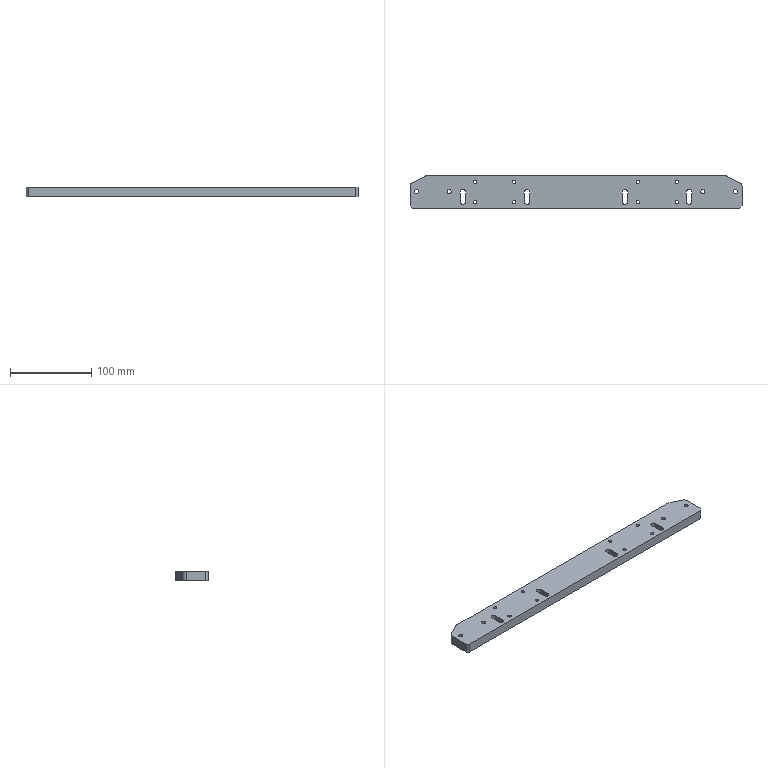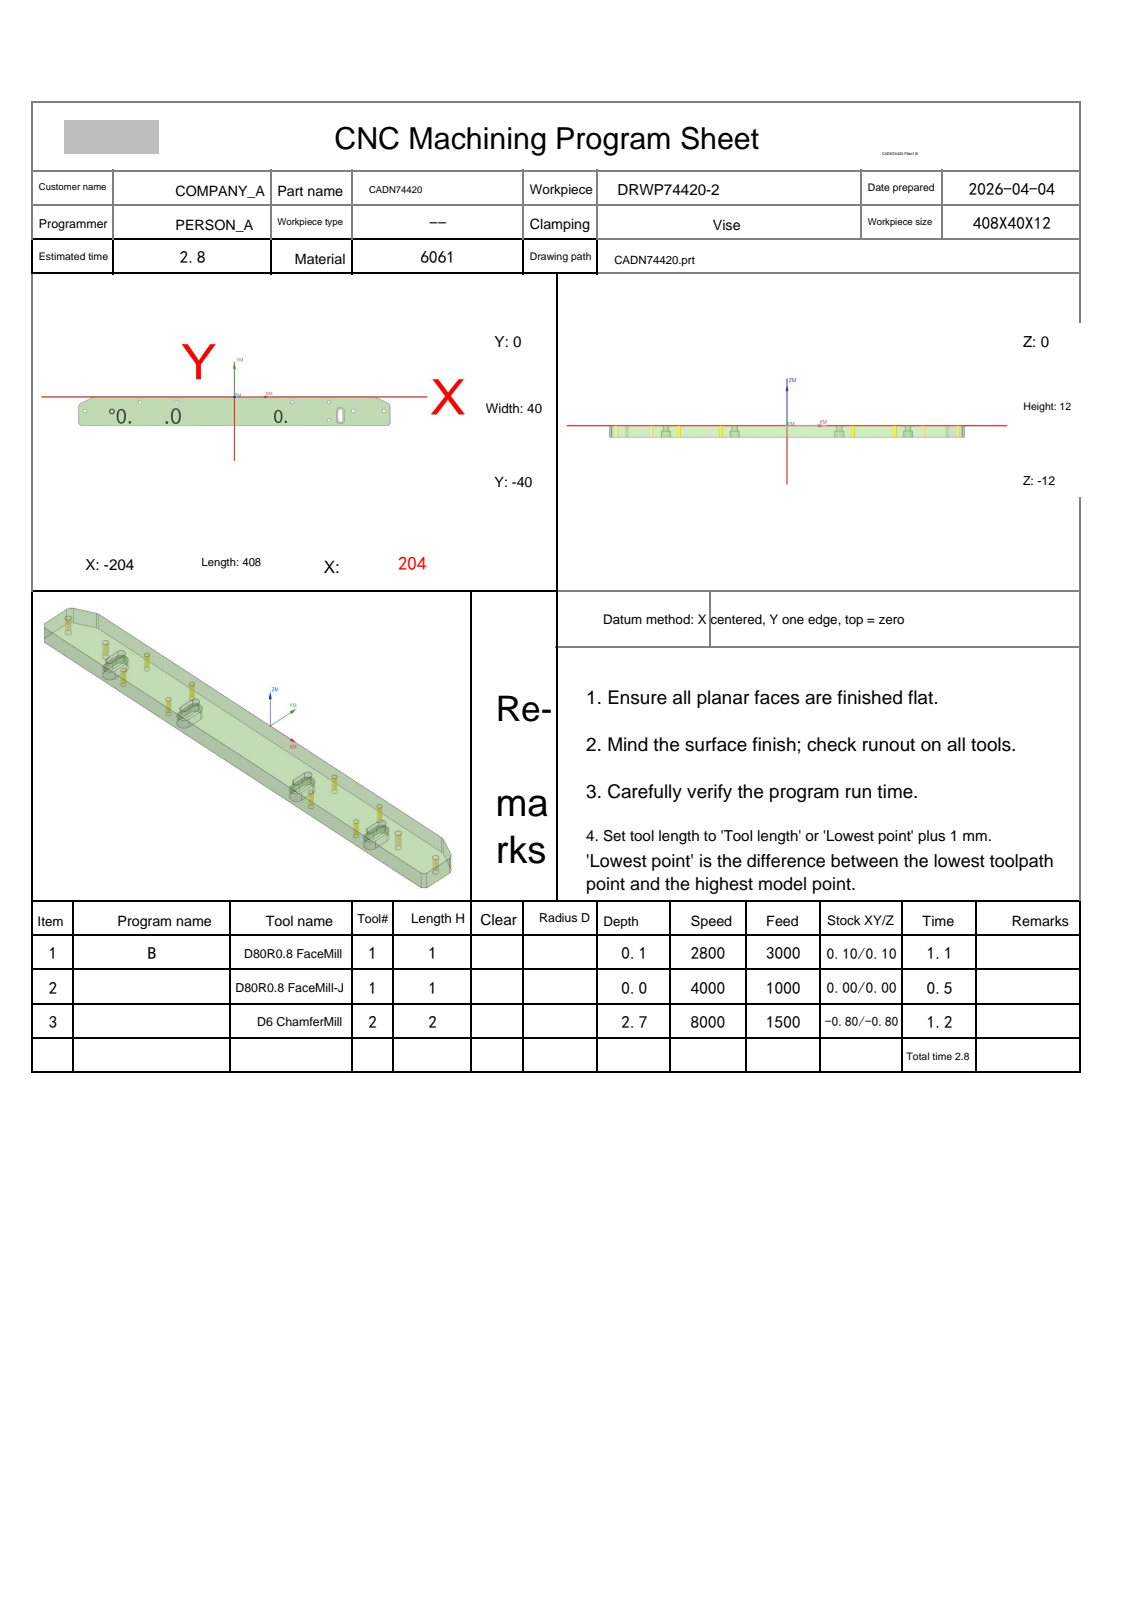NC program | NX | posted by the shop | part box 408 x 40 x 12 mm
Whole program:
%
O0001
(Machine time: 3.33 MIN)
(===Total Tool:2===)
(T1=D80R0.8 FaceMill D=80.  R=0.8  D-  H01 Z=0.    )
(T2=D6 ChamferMill   D=6.   R=0.   D-  H02 Z=-2.7  )
G80 G90 G17 G49 G40
G91 G28 Z0
M01
N1 T01 M06
(D80R0.8 FaceMill  D=80. R=0.8 H=01 ce=0.10 di=0.10)
G00 G90 G54 X-256.097 Y-20. M03 S2800
G43 H01 Z20.
M08
Z4.02
G01 Z2.02 F3000.
X-244.097
X244.097
X256.097
Z4.02
G00 X-256.097
Z3.54
G01 Z1.54
X-244.097
X244.097
X256.097
Z3.54
G00 X-256.097
Z3.06
G01 Z1.06
X-244.097
X244.097
X256.097
Z3.06
G00 X-256.097
Z2.58
G01 Z.58
X-244.097
X244.097
X256.097
Z2.58
G00 Z20.
X-256.097
Z2.1
G01 Z.1
X-244.097
X244.097
X256.097
Z2.1
G00 Z20.
G91 G28 Z0.0
M05
M09
G91 G28 Z0.0
M01
N2 T01 M06
(D80R0.8 FaceMill-J  D=80. R=0.8 H=01 ce=0.00 di=0.00)
G00 G90 G54 X-255.999 Y-20. M03 S4000
G43 H01 Z20.
M08
Z2.
G01 Z0.0 F1000.
X-243.999
X243.999
X255.999
Z2.
G00 Z20.
G91 G28 Z0.0
M05
M09
G91 G28 Z0.0
M01
N3 T02 M06
(D6 ChamferMill  D=6. R=0. H=02 ce=0.00 di=0.00)
G00 G90 G54 X-124. Y-7.5 M03 S8000
G43 H02 Z20.
M08
G98 G81 X-124. Y-7.5 Z-2.7 R3. F1000.
Y-32.5
X-76.
Y-7.5
X76.
Y-32.5
X124.
Y-7.5
G80
G00 Z20.
G00 G90 X-196.232 Y-18.63 M03 S8000
Z20.
Z-.9
G01 Z-1.4 F600.
X-196.4 Y-18.
G03 X-197.9 Y-19.5 I0.0 J-1.5
X-196. Y-21.4 I1.9 J0.0
X-194.1 Y-19.5 I0.0 J1.9
X-196. Y-17.6 I-1.9 J0.0
X-197.9 Y-19.5 I0.0 J-1.9
X-196.4 Y-21. I1.5 J0.0
G01 X-196.232 Y-20.37
Z-.9
G00 Z20.
X-156.232 Y-18.63
Z-.9
G01 Z-1.4
X-156.4 Y-18.
G03 X-157.9 Y-19.5 I0.0 J-1.5
X-156. Y-21.4 I1.9 J0.0
X-154.1 Y-19.5 I0.0 J1.9
X-156. Y-17.6 I-1.9 J0.0
X-157.9 Y-19.5 I0.0 J-1.9
X-156.4 Y-21. I1.5 J0.0
G01 X-156.232 Y-20.37
Z-.9
G00 Z20.
X155.768 Y-18.63
Z-.9
G01 Z-1.4
X155.6 Y-18.
G03 X154.1 Y-19.5 I0.0 J-1.5
X156. Y-21.4 I1.9 J0.0
X157.9 Y-19.5 I0.0 J1.9
X156. Y-17.6 I-1.9 J0.0
X154.1 Y-19.5 I0.0 J-1.9
X155.6 Y-21. I1.5 J0.0
G01 X155.768 Y-20.37
Z-.9
G00 Z20.
X195.768 Y-18.63
Z-.9
G01 Z-1.4
X195.6 Y-18.
G03 X194.1 Y-19.5 I0.0 J-1.5
X196. Y-21.4 I1.9 J0.0
X197.9 Y-19.5 I0.0 J1.9
X196. Y-17.6 I-1.9 J0.0
X194.1 Y-19.5 I0.0 J-1.9
X195.6 Y-21. I1.5 J0.0
G01 X195.768 Y-20.37
Z-.9
G00 Z20.
G00 G90 X.386 Y-41.227 M03 S6500
Z20.
Z.172
G01 Z-1.2 F1500.
G03 X.1 Y-41.027 I-1.286 J-1.532
G01 X.054 Y-40.997
X0.0 Y-41.
X-201.
X-201.259 Y-40.966
X-201.5 Y-40.866
X-201.707 Y-40.707
X-204.707 Y-37.707
X-204.866 Y-37.5
X-204.966 Y-37.259
X-205. Y-37.
Y-13.09
G02 X-201.683 Y-7.724 I6. J0.0
G01 X-185.503 Y.367
G02 X-182.82 Y1. I2.683 J-5.367
G01 X182.82
G02 X185.503 Y.367 I0.0 J-6.
G01 X201.683 Y-7.724
G02 X205. Y-13.09 I-2.683 J-5.367
G01 Y-37.
X204.966 Y-37.259
X204.866 Y-37.5
X204.707 Y-37.707
X201.707 Y-40.707
X201.5 Y-40.866
X201.259 Y-40.966
X201. Y-41.
X0.0
X-.054 Y-40.997
X-.1 Y-41.027
G03 X-.386 Y-41.227 I1. J-1.732
G01 Z.172
G00 Z10.
X-197.315 Y-19.093
Z.284
G01 Z-1.2
G03 X-197.484 Y-19.398 I1.658 J-1.118
G01 X-197.509 Y-19.446
X-197.5 Y-19.5
G03 X-196. Y-21. I1.5 J0.0
X-194.5 Y-19.5 I0.0 J1.5
X-196. Y-18. I-1.5 J0.0
X-197.5 Y-19.5 I0.0 J-1.5
G01 X-197.509 Y-19.554
X-197.484 Y-19.602
G03 X-197.315 Y-19.907 I1.827 J.813
G01 Z.284
G00 Z10.
X-157.315 Y-19.093
Z.284
G01 Z-1.2
G03 X-157.484 Y-19.398 I1.658 J-1.118
G01 X-157.509 Y-19.446
X-157.5 Y-19.5
G03 X-156. Y-21. I1.5 J0.0
X-154.5 Y-19.5 I0.0 J1.5
X-156. Y-18. I-1.5 J0.0
X-157.5 Y-19.5 I0.0 J-1.5
G01 X-157.509 Y-19.554
X-157.484 Y-19.602
G03 X-157.315 Y-19.907 I1.827 J.813
G01 Z.284
G00 Z10.
X-141.073 Y-25.614
Z.172
G01 Z-1.2
G03 X-141.273 Y-25.9 I1.532 J-1.286
G01 X-141.303 Y-25.946
X-141.3 Y-26.
Y-32.
G03 X-139. Y-34.3 I2.3 J0.0
X-136.7 Y-32. I0.0 J2.3
G01 Y-20.
G03 X-139. Y-17.7 I-2.3 J0.0
X-141.3 Y-20. I0.0 J-2.3
G01 Y-26.
X-141.303 Y-26.054
X-141.273 Y-26.1
G03 X-141.073 Y-26.386 I1.732 J1.
G01 Z.172
G00 Z10.
X-123.074 Y-32.912
Z.32
G01 Z-1.2
G03 X-122.914 Y-32.603 I-1.687 J1.075
G01 X-122.89 Y-32.554
X-122.9 Y-32.5
G03 X-124. Y-31.4 I-1.1 J0.0
X-125.1 Y-32.5 I0.0 J-1.1
X-124. Y-33.6 I1.1 J0.0
X-122.9 Y-32.5 I0.0 J1.1
G01 X-122.89 Y-32.446
X-122.914 Y-32.397
G03 X-123.074 Y-32.088 I-1.848 J-.765
G01 Z.32
G00 Z10.
Y-7.912
Z.32
G01 Z-1.2
G03 X-122.914 Y-7.603 I-1.687 J1.075
G01 X-122.89 Y-7.554
X-122.9 Y-7.5
G03 X-124. Y-6.4 I-1.1 J0.0
X-125.1 Y-7.5 I0.0 J-1.1
X-124. Y-8.6 I1.1 J0.0
X-122.9 Y-7.5 I0.0 J1.1
G01 X-122.89 Y-7.446
X-122.914 Y-7.397
G03 X-123.074 Y-7.088 I-1.848 J-.765
G01 Z.32
G00 Z10.
X-75.074 Y-7.912
Z.32
G01 Z-1.2
G03 X-74.914 Y-7.603 I-1.687 J1.075
G01 X-74.89 Y-7.554
X-74.9 Y-7.5
G03 X-76. Y-6.4 I-1.1 J0.0
X-77.1 Y-7.5 I0.0 J-1.1
X-76. Y-8.6 I1.1 J0.0
X-74.9 Y-7.5 I0.0 J1.1
G01 X-74.89 Y-7.446
X-74.914 Y-7.397
G03 X-75.074 Y-7.088 I-1.848 J-.765
G01 Z.32
G00 Z10.
Y-32.912
Z.32
G01 Z-1.2
G03 X-74.914 Y-32.603 I-1.687 J1.075
G01 X-74.89 Y-32.554
X-74.9 Y-32.5
G03 X-76. Y-31.4 I-1.1 J0.0
X-77.1 Y-32.5 I0.0 J-1.1
X-76. Y-33.6 I1.1 J0.0
X-74.9 Y-32.5 I0.0 J1.1
G01 X-74.89 Y-32.446
X-74.914 Y-32.397
G03 X-75.074 Y-32.088 I-1.848 J-.765
G01 Z.32
G00 Z10.
X-62.073 Y-25.614
Z.172
G01 Z-1.2
G03 X-62.273 Y-25.9 I1.532 J-1.286
G01 X-62.303 Y-25.946
X-62.3 Y-26.
Y-32.
G03 X-60. Y-34.3 I2.3 J0.0
X-57.7 Y-32. I0.0 J2.3
G01 Y-20.
G03 X-60. Y-17.7 I-2.3 J0.0
X-62.3 Y-20. I0.0 J-2.3
G01 Y-26.
X-62.303 Y-26.054
X-62.273 Y-26.1
G03 X-62.073 Y-26.386 I1.732 J1.
G01 Z.172
G00 Z10.
X57.927 Y-25.614
Z.172
G01 Z-1.2
G03 X57.727 Y-25.9 I1.532 J-1.286
G01 X57.697 Y-25.946
X57.7 Y-26.
Y-32.
G03 X60. Y-34.3 I2.3 J0.0
X62.3 Y-32. I0.0 J2.3
G01 Y-20.
G03 X60. Y-17.7 I-2.3 J0.0
X57.7 Y-20. I0.0 J-2.3
G01 Y-26.
X57.697 Y-26.054
X57.727 Y-26.1
G03 X57.927 Y-26.386 I1.732 J1.
G01 Z.172
G00 Z10.
X76.926 Y-32.912
Z.32
G01 Z-1.2
G03 X77.086 Y-32.603 I-1.687 J1.075
G01 X77.11 Y-32.554
X77.1 Y-32.5
G03 X76. Y-31.4 I-1.1 J0.0
X74.9 Y-32.5 I0.0 J-1.1
X76. Y-33.6 I1.1 J0.0
X77.1 Y-32.5 I0.0 J1.1
G01 X77.11 Y-32.446
X77.086 Y-32.397
G03 X76.926 Y-32.088 I-1.848 J-.765
G01 Z.32
G00 Z10.
Y-7.912
Z.32
G01 Z-1.2
G03 X77.086 Y-7.603 I-1.687 J1.075
G01 X77.11 Y-7.554
X77.1 Y-7.5
G03 X76. Y-6.4 I-1.1 J0.0
X74.9 Y-7.5 I0.0 J-1.1
X76. Y-8.6 I1.1 J0.0
X77.1 Y-7.5 I0.0 J1.1
G01 X77.11 Y-7.446
X77.086 Y-7.397
G03 X76.926 Y-7.088 I-1.848 J-.765
G01 Z.32
G00 Z10.
X124.926 Y-7.912
Z.32
G01 Z-1.2
G03 X125.086 Y-7.603 I-1.687 J1.075
G01 X125.11 Y-7.554
X125.1 Y-7.5
G03 X124. Y-6.4 I-1.1 J0.0
X122.9 Y-7.5 I0.0 J-1.1
X124. Y-8.6 I1.1 J0.0
X125.1 Y-7.5 I0.0 J1.1
G01 X125.11 Y-7.446
X125.086 Y-7.397
G03 X124.926 Y-7.088 I-1.848 J-.765
G01 Z.32
G00 Z10.
Y-32.912
Z.32
G01 Z-1.2
G03 X125.086 Y-32.603 I-1.687 J1.075
G01 X125.11 Y-32.554
X125.1 Y-32.5
G03 X124. Y-31.4 I-1.1 J0.0
X122.9 Y-32.5 I0.0 J-1.1
X124. Y-33.6 I1.1 J0.0
X125.1 Y-32.5 I0.0 J1.1
G01 X125.11 Y-32.446
X125.086 Y-32.397
G03 X124.926 Y-32.088 I-1.848 J-.765
G01 Z.32
G00 Z10.
X136.927 Y-25.614
Z.172
G01 Z-1.2
G03 X136.727 Y-25.9 I1.532 J-1.286
G01 X136.697 Y-25.946
X136.7 Y-26.
Y-32.
G03 X139. Y-34.3 I2.3 J0.0
X141.3 Y-32. I0.0 J2.3
G01 Y-20.
G03 X139. Y-17.7 I-2.3 J0.0
X136.7 Y-20. I0.0 J-2.3
G01 Y-26.
X136.697 Y-26.054
X136.727 Y-26.1
G03 X136.927 Y-26.386 I1.732 J1.
G01 Z.172
G00 Z10.
X154.685 Y-19.093
Z.284
G01 Z-1.2
G03 X154.516 Y-19.398 I1.658 J-1.118
G01 X154.491 Y-19.446
X154.5 Y-19.5
G03 X156. Y-21. I1.5 J0.0
X157.5 Y-19.5 I0.0 J1.5
X156. Y-18. I-1.5 J0.0
X154.5 Y-19.5 I0.0 J-1.5
G01 X154.491 Y-19.554
X154.516 Y-19.602
G03 X154.685 Y-19.907 I1.827 J.813
G01 Z.284
G00 Z10.
X194.685 Y-19.093
Z.284
G01 Z-1.2
G03 X194.516 Y-19.398 I1.658 J-1.118
G01 X194.491 Y-19.446
X194.5 Y-19.5
G03 X196. Y-21. I1.5 J0.0
X197.5 Y-19.5 I0.0 J1.5
X196. Y-18. I-1.5 J0.0
X194.5 Y-19.5 I0.0 J-1.5
G01 X194.491 Y-19.554
X194.516 Y-19.602
G03 X194.685 Y-19.907 I1.827 J.813
G01 Z.284
G00 Z20.
M05
M09
G91 G28 Z0.0
G91 G28 Y0.0
M30
%